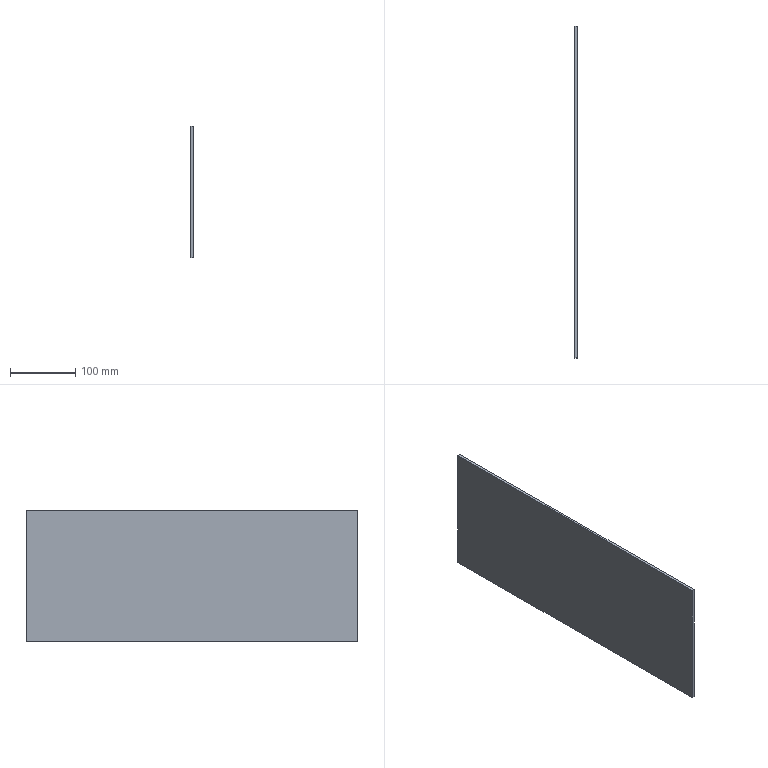Part | STEP file | 1 solid | 6 faces | box 4 x 509.2 x 201.1 mm | volume 409600 mm3 | plane 6
STEP:
#1=CARTESIAN_POINT('',(0.,0.,0.));
#2=DIRECTION('',(0.,0.,1.));
#3=DIRECTION('',(1.,0.,0.));
#4=AXIS2_PLACEMENT_3D('',#1,#2,#3);
#5=CARTESIAN_POINT('',(761.,4665.,1648.394));
#6=VERTEX_POINT('',#5);
#7=CARTESIAN_POINT('',(761.,4665.,1447.294));
#8=VERTEX_POINT('',#7);
#9=CARTESIAN_POINT('',(761.,4665.,1648.394));
#10=DIRECTION('',(0.,0.,-1.));
#11=VECTOR('',#10,1.);
#12=LINE('',#9,#11);
#13=CARTESIAN_POINT('',(765.,4665.,1447.294));
#14=DIRECTION('',(0.,-1.,0.));
#15=DIRECTION('',(0.,0.,-1.));
#16=AXIS2_PLACEMENT_3D('',#13,#14,#15);
#17=PLANE('',#16);
#18=CARTESIAN_POINT('',(-201.1,-4.));
#19=DIRECTION('',(1.,0.));
#20=VECTOR('',#19,1.);
#21=LINE('',#18,#20);
#22=(GEOMETRIC_REPRESENTATION_CONTEXT(2)PARAMETRIC_REPRESENTATION_CONTEXT()REPRESENTATION_CONTEXT('',''));
#23=DEFINITIONAL_REPRESENTATION('',(#21),#22);
#24=PCURVE('',#17,#23);
#25=CARTESIAN_POINT('',(761.,0.,0.));
#26=DIRECTION('',(-1.,0.,0.));
#27=DIRECTION('',(0.,0.,1.));
#28=AXIS2_PLACEMENT_3D('',#25,#26,#27);
#29=PLANE('',#28);
#30=CARTESIAN_POINT('',(1648.394,4665.));
#31=DIRECTION('',(-1.,0.));
#32=VECTOR('',#31,1.);
#33=LINE('',#30,#32);
#34=(GEOMETRIC_REPRESENTATION_CONTEXT(2)PARAMETRIC_REPRESENTATION_CONTEXT()REPRESENTATION_CONTEXT('',''));
#35=DEFINITIONAL_REPRESENTATION('',(#33),#34);
#36=PCURVE('',#29,#35);
#37=SURFACE_CURVE('',#12,(#24,#36),.PCURVE_S1.);
#38=EDGE_CURVE('',#6,#8,#37,.T.);
#39=ORIENTED_EDGE('',*,*,#38,.F.);
#40=CARTESIAN_POINT('',(765.,4665.,1648.394));
#41=VERTEX_POINT('',#40);
#42=CARTESIAN_POINT('',(761.,4665.,1648.394));
#43=DIRECTION('',(1.,0.,0.));
#44=VECTOR('',#43,1.);
#45=LINE('',#42,#44);
#46=CARTESIAN_POINT('',(-201.1,-4.));
#47=DIRECTION('',(0.,1.));
#48=VECTOR('',#47,1.);
#49=LINE('',#46,#48);
#50=(GEOMETRIC_REPRESENTATION_CONTEXT(2)PARAMETRIC_REPRESENTATION_CONTEXT()REPRESENTATION_CONTEXT('',''));
#51=DEFINITIONAL_REPRESENTATION('',(#49),#50);
#52=PCURVE('',#17,#51);
#53=CARTESIAN_POINT('',(765.,4665.,1648.394));
#54=DIRECTION('',(0.,0.,1.));
#55=DIRECTION('',(1.,0.,0.));
#56=AXIS2_PLACEMENT_3D('',#53,#54,#55);
#57=PLANE('',#56);
#58=CARTESIAN_POINT('',(-4.,0.));
#59=DIRECTION('',(1.,0.));
#60=VECTOR('',#59,1.);
#61=LINE('',#58,#60);
#62=(GEOMETRIC_REPRESENTATION_CONTEXT(2)PARAMETRIC_REPRESENTATION_CONTEXT()REPRESENTATION_CONTEXT('',''));
#63=DEFINITIONAL_REPRESENTATION('',(#61),#62);
#64=PCURVE('',#57,#63);
#65=SURFACE_CURVE('',#45,(#52,#64),.PCURVE_S1.);
#66=EDGE_CURVE('',#6,#41,#65,.T.);
#67=ORIENTED_EDGE('',*,*,#66,.T.);
#68=CARTESIAN_POINT('',(765.,4665.,1447.294));
#69=VERTEX_POINT('',#68);
#70=CARTESIAN_POINT('',(765.,4665.,1648.394));
#71=DIRECTION('',(0.,0.,-1.));
#72=VECTOR('',#71,1.);
#73=LINE('',#70,#72);
#74=CARTESIAN_POINT('',(-201.1,0.));
#75=DIRECTION('',(1.,0.));
#76=VECTOR('',#75,1.);
#77=LINE('',#74,#76);
#78=(GEOMETRIC_REPRESENTATION_CONTEXT(2)PARAMETRIC_REPRESENTATION_CONTEXT()REPRESENTATION_CONTEXT('',''));
#79=DEFINITIONAL_REPRESENTATION('',(#77),#78);
#80=PCURVE('',#17,#79);
#81=CARTESIAN_POINT('',(765.,0.,0.));
#82=DIRECTION('',(-1.,0.,0.));
#83=DIRECTION('',(0.,0.,1.));
#84=AXIS2_PLACEMENT_3D('',#81,#82,#83);
#85=PLANE('',#84);
#86=CARTESIAN_POINT('',(1648.394,4665.));
#87=DIRECTION('',(-1.,0.));
#88=VECTOR('',#87,1.);
#89=LINE('',#86,#88);
#90=(GEOMETRIC_REPRESENTATION_CONTEXT(2)PARAMETRIC_REPRESENTATION_CONTEXT()REPRESENTATION_CONTEXT('',''));
#91=DEFINITIONAL_REPRESENTATION('',(#89),#90);
#92=PCURVE('',#85,#91);
#93=SURFACE_CURVE('',#73,(#80,#92),.PCURVE_S1.);
#94=EDGE_CURVE('',#41,#69,#93,.T.);
#95=ORIENTED_EDGE('',*,*,#94,.T.);
#96=CARTESIAN_POINT('',(761.,4665.,1447.294));
#97=DIRECTION('',(1.,0.,0.));
#98=VECTOR('',#97,1.);
#99=LINE('',#96,#98);
#100=CARTESIAN_POINT('',(0.,-4.));
#101=DIRECTION('',(0.,1.));
#102=VECTOR('',#101,1.);
#103=LINE('',#100,#102);
#104=(GEOMETRIC_REPRESENTATION_CONTEXT(2)PARAMETRIC_REPRESENTATION_CONTEXT()REPRESENTATION_CONTEXT('',''));
#105=DEFINITIONAL_REPRESENTATION('',(#103),#104);
#106=PCURVE('',#17,#105);
#107=CARTESIAN_POINT('',(765.,5174.2,1447.294));
#108=DIRECTION('',(0.,0.,-1.));
#109=DIRECTION('',(-1.,0.,0.));
#110=AXIS2_PLACEMENT_3D('',#107,#108,#109);
#111=PLANE('',#110);
#112=CARTESIAN_POINT('',(4.,-509.2));
#113=DIRECTION('',(-1.,0.));
#114=VECTOR('',#113,1.);
#115=LINE('',#112,#114);
#116=(GEOMETRIC_REPRESENTATION_CONTEXT(2)PARAMETRIC_REPRESENTATION_CONTEXT()REPRESENTATION_CONTEXT('',''));
#117=DEFINITIONAL_REPRESENTATION('',(#115),#116);
#118=PCURVE('',#111,#117);
#119=SURFACE_CURVE('',#99,(#106,#118),.PCURVE_S1.);
#120=EDGE_CURVE('',#8,#69,#119,.T.);
#121=ORIENTED_EDGE('',*,*,#120,.F.);
#122=EDGE_LOOP('',(#39,#67,#95,#121));
#123=FACE_BOUND('',#122,.F.);
#124=ADVANCED_FACE('',(#123),#17,.T.);
#125=ORIENTED_EDGE('',*,*,#38,.T.);
#126=CARTESIAN_POINT('',(761.,5174.2,1447.294));
#127=VERTEX_POINT('',#126);
#128=CARTESIAN_POINT('',(761.,4665.,1447.294));
#129=DIRECTION('',(0.,1.,0.));
#130=VECTOR('',#129,1.);
#131=LINE('',#128,#130);
#132=CARTESIAN_POINT('',(1447.294,4665.));
#133=DIRECTION('',(0.,1.));
#134=VECTOR('',#133,1.);
#135=LINE('',#132,#134);
#136=(GEOMETRIC_REPRESENTATION_CONTEXT(2)PARAMETRIC_REPRESENTATION_CONTEXT()REPRESENTATION_CONTEXT('',''));
#137=DEFINITIONAL_REPRESENTATION('',(#135),#136);
#138=PCURVE('',#29,#137);
#139=CARTESIAN_POINT('',(4.,-509.2));
#140=DIRECTION('',(0.,1.));
#141=VECTOR('',#140,1.);
#142=LINE('',#139,#141);
#143=(GEOMETRIC_REPRESENTATION_CONTEXT(2)PARAMETRIC_REPRESENTATION_CONTEXT()REPRESENTATION_CONTEXT('',''));
#144=DEFINITIONAL_REPRESENTATION('',(#142),#143);
#145=PCURVE('',#111,#144);
#146=SURFACE_CURVE('',#131,(#138,#145),.PCURVE_S1.);
#147=EDGE_CURVE('',#8,#127,#146,.T.);
#148=ORIENTED_EDGE('',*,*,#147,.T.);
#149=CARTESIAN_POINT('',(761.,5174.2,1648.394));
#150=VERTEX_POINT('',#149);
#151=CARTESIAN_POINT('',(761.,5174.2,1447.294));
#152=DIRECTION('',(0.,0.,1.));
#153=VECTOR('',#152,1.);
#154=LINE('',#151,#153);
#155=CARTESIAN_POINT('',(1447.294,5174.2));
#156=DIRECTION('',(1.,0.));
#157=VECTOR('',#156,1.);
#158=LINE('',#155,#157);
#159=(GEOMETRIC_REPRESENTATION_CONTEXT(2)PARAMETRIC_REPRESENTATION_CONTEXT()REPRESENTATION_CONTEXT('',''));
#160=DEFINITIONAL_REPRESENTATION('',(#158),#159);
#161=PCURVE('',#29,#160);
#162=CARTESIAN_POINT('',(765.,5174.2,1648.394));
#163=DIRECTION('',(0.,1.,0.));
#164=DIRECTION('',(0.,0.,1.));
#165=AXIS2_PLACEMENT_3D('',#162,#163,#164);
#166=PLANE('',#165);
#167=CARTESIAN_POINT('',(-201.1,-4.));
#168=DIRECTION('',(1.,0.));
#169=VECTOR('',#168,1.);
#170=LINE('',#167,#169);
#171=(GEOMETRIC_REPRESENTATION_CONTEXT(2)PARAMETRIC_REPRESENTATION_CONTEXT()REPRESENTATION_CONTEXT('',''));
#172=DEFINITIONAL_REPRESENTATION('',(#170),#171);
#173=PCURVE('',#166,#172);
#174=SURFACE_CURVE('',#154,(#161,#173),.PCURVE_S1.);
#175=EDGE_CURVE('',#127,#150,#174,.T.);
#176=ORIENTED_EDGE('',*,*,#175,.T.);
#177=CARTESIAN_POINT('',(761.,5174.2,1648.394));
#178=DIRECTION('',(0.,-1.,0.));
#179=VECTOR('',#178,1.);
#180=LINE('',#177,#179);
#181=CARTESIAN_POINT('',(1648.394,5174.2));
#182=DIRECTION('',(0.,-1.));
#183=VECTOR('',#182,1.);
#184=LINE('',#181,#183);
#185=(GEOMETRIC_REPRESENTATION_CONTEXT(2)PARAMETRIC_REPRESENTATION_CONTEXT()REPRESENTATION_CONTEXT('',''));
#186=DEFINITIONAL_REPRESENTATION('',(#184),#185);
#187=PCURVE('',#29,#186);
#188=CARTESIAN_POINT('',(-4.,509.2));
#189=DIRECTION('',(0.,-1.));
#190=VECTOR('',#189,1.);
#191=LINE('',#188,#190);
#192=(GEOMETRIC_REPRESENTATION_CONTEXT(2)PARAMETRIC_REPRESENTATION_CONTEXT()REPRESENTATION_CONTEXT('',''));
#193=DEFINITIONAL_REPRESENTATION('',(#191),#192);
#194=PCURVE('',#57,#193);
#195=SURFACE_CURVE('',#180,(#187,#194),.PCURVE_S1.);
#196=EDGE_CURVE('',#150,#6,#195,.T.);
#197=ORIENTED_EDGE('',*,*,#196,.T.);
#198=EDGE_LOOP('',(#125,#148,#176,#197));
#199=FACE_BOUND('',#198,.F.);
#200=ADVANCED_FACE('',(#199),#29,.T.);
#201=ORIENTED_EDGE('',*,*,#147,.F.);
#202=ORIENTED_EDGE('',*,*,#120,.T.);
#203=CARTESIAN_POINT('',(765.,5174.2,1447.294));
#204=VERTEX_POINT('',#203);
#205=CARTESIAN_POINT('',(765.,4665.,1447.294));
#206=DIRECTION('',(0.,1.,0.));
#207=VECTOR('',#206,1.);
#208=LINE('',#205,#207);
#209=CARTESIAN_POINT('',(0.,-509.2));
#210=DIRECTION('',(0.,1.));
#211=VECTOR('',#210,1.);
#212=LINE('',#209,#211);
#213=(GEOMETRIC_REPRESENTATION_CONTEXT(2)PARAMETRIC_REPRESENTATION_CONTEXT()REPRESENTATION_CONTEXT('',''));
#214=DEFINITIONAL_REPRESENTATION('',(#212),#213);
#215=PCURVE('',#111,#214);
#216=CARTESIAN_POINT('',(1447.294,4665.));
#217=DIRECTION('',(0.,1.));
#218=VECTOR('',#217,1.);
#219=LINE('',#216,#218);
#220=(GEOMETRIC_REPRESENTATION_CONTEXT(2)PARAMETRIC_REPRESENTATION_CONTEXT()REPRESENTATION_CONTEXT('',''));
#221=DEFINITIONAL_REPRESENTATION('',(#219),#220);
#222=PCURVE('',#85,#221);
#223=SURFACE_CURVE('',#208,(#215,#222),.PCURVE_S1.);
#224=EDGE_CURVE('',#69,#204,#223,.T.);
#225=ORIENTED_EDGE('',*,*,#224,.T.);
#226=CARTESIAN_POINT('',(761.,5174.2,1447.294));
#227=DIRECTION('',(1.,0.,0.));
#228=VECTOR('',#227,1.);
#229=LINE('',#226,#228);
#230=CARTESIAN_POINT('',(4.,0.));
#231=DIRECTION('',(-1.,0.));
#232=VECTOR('',#231,1.);
#233=LINE('',#230,#232);
#234=(GEOMETRIC_REPRESENTATION_CONTEXT(2)PARAMETRIC_REPRESENTATION_CONTEXT()REPRESENTATION_CONTEXT('',''));
#235=DEFINITIONAL_REPRESENTATION('',(#233),#234);
#236=PCURVE('',#111,#235);
#237=CARTESIAN_POINT('',(-201.1,-4.));
#238=DIRECTION('',(0.,1.));
#239=VECTOR('',#238,1.);
#240=LINE('',#237,#239);
#241=(GEOMETRIC_REPRESENTATION_CONTEXT(2)PARAMETRIC_REPRESENTATION_CONTEXT()REPRESENTATION_CONTEXT('',''));
#242=DEFINITIONAL_REPRESENTATION('',(#240),#241);
#243=PCURVE('',#166,#242);
#244=SURFACE_CURVE('',#229,(#236,#243),.PCURVE_S1.);
#245=EDGE_CURVE('',#127,#204,#244,.T.);
#246=ORIENTED_EDGE('',*,*,#245,.F.);
#247=EDGE_LOOP('',(#201,#202,#225,#246));
#248=FACE_BOUND('',#247,.F.);
#249=ADVANCED_FACE('',(#248),#111,.T.);
#250=ORIENTED_EDGE('',*,*,#94,.F.);
#251=CARTESIAN_POINT('',(765.,5174.2,1648.394));
#252=VERTEX_POINT('',#251);
#253=CARTESIAN_POINT('',(765.,5174.2,1648.394));
#254=DIRECTION('',(0.,-1.,0.));
#255=VECTOR('',#254,1.);
#256=LINE('',#253,#255);
#257=CARTESIAN_POINT('',(1648.394,5174.2));
#258=DIRECTION('',(0.,-1.));
#259=VECTOR('',#258,1.);
#260=LINE('',#257,#259);
#261=(GEOMETRIC_REPRESENTATION_CONTEXT(2)PARAMETRIC_REPRESENTATION_CONTEXT()REPRESENTATION_CONTEXT('',''));
#262=DEFINITIONAL_REPRESENTATION('',(#260),#261);
#263=PCURVE('',#85,#262);
#264=CARTESIAN_POINT('',(0.,509.2));
#265=DIRECTION('',(0.,-1.));
#266=VECTOR('',#265,1.);
#267=LINE('',#264,#266);
#268=(GEOMETRIC_REPRESENTATION_CONTEXT(2)PARAMETRIC_REPRESENTATION_CONTEXT()REPRESENTATION_CONTEXT('',''));
#269=DEFINITIONAL_REPRESENTATION('',(#267),#268);
#270=PCURVE('',#57,#269);
#271=SURFACE_CURVE('',#256,(#263,#270),.PCURVE_S1.);
#272=EDGE_CURVE('',#252,#41,#271,.T.);
#273=ORIENTED_EDGE('',*,*,#272,.F.);
#274=CARTESIAN_POINT('',(765.,5174.2,1447.294));
#275=DIRECTION('',(0.,0.,1.));
#276=VECTOR('',#275,1.);
#277=LINE('',#274,#276);
#278=CARTESIAN_POINT('',(1447.294,5174.2));
#279=DIRECTION('',(1.,0.));
#280=VECTOR('',#279,1.);
#281=LINE('',#278,#280);
#282=(GEOMETRIC_REPRESENTATION_CONTEXT(2)PARAMETRIC_REPRESENTATION_CONTEXT()REPRESENTATION_CONTEXT('',''));
#283=DEFINITIONAL_REPRESENTATION('',(#281),#282);
#284=PCURVE('',#85,#283);
#285=CARTESIAN_POINT('',(-201.1,0.));
#286=DIRECTION('',(1.,0.));
#287=VECTOR('',#286,1.);
#288=LINE('',#285,#287);
#289=(GEOMETRIC_REPRESENTATION_CONTEXT(2)PARAMETRIC_REPRESENTATION_CONTEXT()REPRESENTATION_CONTEXT('',''));
#290=DEFINITIONAL_REPRESENTATION('',(#288),#289);
#291=PCURVE('',#166,#290);
#292=SURFACE_CURVE('',#277,(#284,#291),.PCURVE_S1.);
#293=EDGE_CURVE('',#204,#252,#292,.T.);
#294=ORIENTED_EDGE('',*,*,#293,.F.);
#295=ORIENTED_EDGE('',*,*,#224,.F.);
#296=EDGE_LOOP('',(#250,#273,#294,#295));
#297=FACE_BOUND('',#296,.F.);
#298=ADVANCED_FACE('',(#297),#85,.F.);
#299=ORIENTED_EDGE('',*,*,#196,.F.);
#300=CARTESIAN_POINT('',(761.,5174.2,1648.394));
#301=DIRECTION('',(1.,0.,0.));
#302=VECTOR('',#301,1.);
#303=LINE('',#300,#302);
#304=CARTESIAN_POINT('',(-4.,509.2));
#305=DIRECTION('',(1.,0.));
#306=VECTOR('',#305,1.);
#307=LINE('',#304,#306);
#308=(GEOMETRIC_REPRESENTATION_CONTEXT(2)PARAMETRIC_REPRESENTATION_CONTEXT()REPRESENTATION_CONTEXT('',''));
#309=DEFINITIONAL_REPRESENTATION('',(#307),#308);
#310=PCURVE('',#57,#309);
#311=CARTESIAN_POINT('',(0.,-4.));
#312=DIRECTION('',(0.,1.));
#313=VECTOR('',#312,1.);
#314=LINE('',#311,#313);
#315=(GEOMETRIC_REPRESENTATION_CONTEXT(2)PARAMETRIC_REPRESENTATION_CONTEXT()REPRESENTATION_CONTEXT('',''));
#316=DEFINITIONAL_REPRESENTATION('',(#314),#315);
#317=PCURVE('',#166,#316);
#318=SURFACE_CURVE('',#303,(#310,#317),.PCURVE_S1.);
#319=EDGE_CURVE('',#150,#252,#318,.T.);
#320=ORIENTED_EDGE('',*,*,#319,.T.);
#321=ORIENTED_EDGE('',*,*,#272,.T.);
#322=ORIENTED_EDGE('',*,*,#66,.F.);
#323=EDGE_LOOP('',(#299,#320,#321,#322));
#324=FACE_BOUND('',#323,.F.);
#325=ADVANCED_FACE('',(#324),#57,.T.);
#326=ORIENTED_EDGE('',*,*,#175,.F.);
#327=ORIENTED_EDGE('',*,*,#245,.T.);
#328=ORIENTED_EDGE('',*,*,#293,.T.);
#329=ORIENTED_EDGE('',*,*,#319,.F.);
#330=EDGE_LOOP('',(#326,#327,#328,#329));
#331=FACE_BOUND('',#330,.F.);
#332=ADVANCED_FACE('',(#331),#166,.T.);
#333=CLOSED_SHELL('',(#124,#200,#249,#298,#325,#332));
#334=MANIFOLD_SOLID_BREP('',#333);
#335=(LENGTH_UNIT()NAMED_UNIT(*)SI_UNIT(.MILLI.,.METRE.));
#336=UNCERTAINTY_MEASURE_WITH_UNIT(LENGTH_MEASURE(0.0000001),#335,'','');
#337=(NAMED_UNIT(*)PLANE_ANGLE_UNIT()SI_UNIT($,.RADIAN.));
#338=(NAMED_UNIT(*)SI_UNIT($,.STERADIAN.)SOLID_ANGLE_UNIT());
#339=(GEOMETRIC_REPRESENTATION_CONTEXT(3)GLOBAL_UNCERTAINTY_ASSIGNED_CONTEXT((#336))GLOBAL_UNIT_ASSIGNED_CONTEXT((#335,#337,#338))REPRESENTATION_CONTEXT('',''));
#340=ADVANCED_BREP_SHAPE_REPRESENTATION('',(#4,#334),#339);